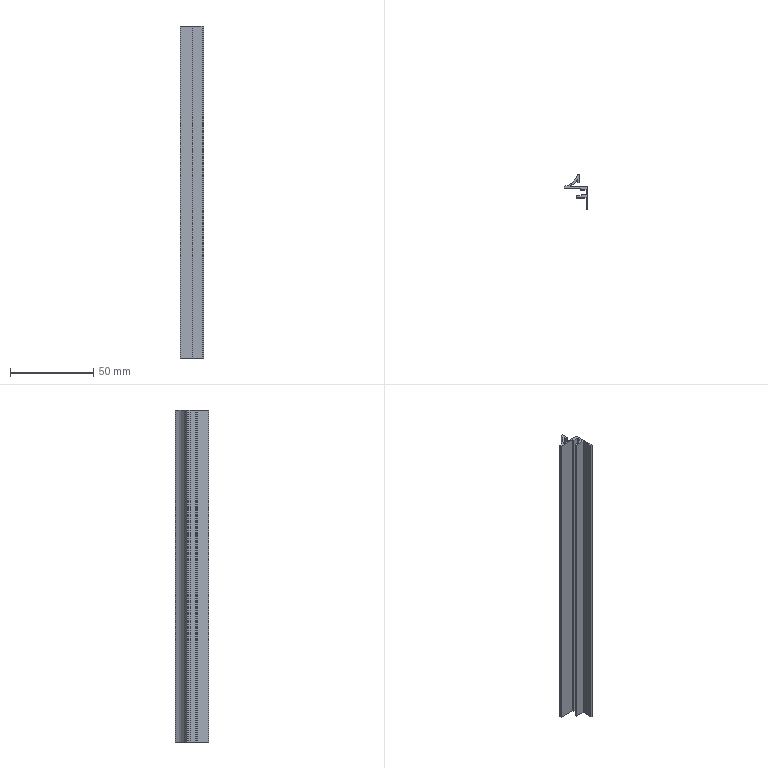Part | SolidWorks | features BaseBody 1, ICE 1, MoveFace 1 | 1 solid | 27 faces | box 14 x 20.3 x 199 mm | volume 10132 mm3 | plane 20 | cylinder 7 | commonest cylinder face diameters 0.387 x2 0.8 x2 0.4 x1 20 x1 22 x1
STEP:
#1=CARTESIAN_POINT('',(-5.304,-0.625,200.));
#2=VERTEX_POINT('',#1);
#3=CARTESIAN_POINT('',(-5.449,-0.8125,200.));
#4=VERTEX_POINT('',#3);
#5=CARTESIAN_POINT('',(-5.255,-0.8125,200.));
#6=DIRECTION('',(0.,0.,1.));
#7=DIRECTION('',(-1.,0.,0.));
#8=AXIS2_PLACEMENT_3D('',#5,#6,#7);
#9=CIRCLE('',#8,0.1937);
#10=EDGE_CURVE('',#2,#4,#9,.T.);
#11=ORIENTED_EDGE('',*,*,#10,.T.);
#12=CARTESIAN_POINT('',(-5.449,-0.8125,1.));
#13=VERTEX_POINT('',#12);
#14=CARTESIAN_POINT('',(-5.449,-0.8125,230.));
#15=DIRECTION('',(0.,0.,-1.));
#16=VECTOR('',#15,1000.);
#17=LINE('',#14,#16);
#18=EDGE_CURVE('',#4,#13,#17,.T.);
#19=ORIENTED_EDGE('',*,*,#18,.T.);
#20=CARTESIAN_POINT('',(-5.304,-0.625,1.));
#21=VERTEX_POINT('',#20);
#22=CARTESIAN_POINT('',(-5.255,-0.8125,1.));
#23=DIRECTION('',(0.,0.,-1.));
#24=DIRECTION('',(1.,0.,0.));
#25=AXIS2_PLACEMENT_3D('',#22,#23,#24);
#26=CIRCLE('',#25,0.1937);
#27=EDGE_CURVE('',#13,#21,#26,.T.);
#28=ORIENTED_EDGE('',*,*,#27,.T.);
#29=CARTESIAN_POINT('',(-5.304,-0.625,230.));
#30=DIRECTION('',(0.,0.,-1.));
#31=VECTOR('',#30,1000.);
#32=LINE('',#29,#31);
#33=EDGE_CURVE('',#2,#21,#32,.T.);
#34=ORIENTED_EDGE('',*,*,#33,.F.);
#35=EDGE_LOOP('',(#11,#19,#28,#34));
#36=FACE_OUTER_BOUND('',#35,.T.);
#37=CARTESIAN_POINT('',(-5.255,-0.8125,230.));
#38=DIRECTION('',(0.,0.,-1.));
#39=DIRECTION('',(-1.,0.,0.));
#40=AXIS2_PLACEMENT_3D('',#37,#38,#39);
#41=CYLINDRICAL_SURFACE('',#40,0.1937);
#42=ADVANCED_FACE('',(#36),#41,.F.);
#43=CARTESIAN_POINT('',(5.,-1.,1.));
#44=VERTEX_POINT('',#43);
#45=CARTESIAN_POINT('',(5.,-14.3,1.));
#46=VERTEX_POINT('',#45);
#47=CARTESIAN_POINT('',(5.,29.623,1.));
#48=DIRECTION('',(0.,-1.,0.));
#49=VECTOR('',#48,1000.);
#50=LINE('',#47,#49);
#51=EDGE_CURVE('',#44,#46,#50,.T.);
#52=ORIENTED_EDGE('',*,*,#51,.F.);
#53=CARTESIAN_POINT('',(5.,-1.,200.));
#54=VERTEX_POINT('',#53);
#55=CARTESIAN_POINT('',(5.,-1.,230.));
#56=DIRECTION('',(0.,0.,-1.));
#57=VECTOR('',#56,1000.);
#58=LINE('',#55,#57);
#59=EDGE_CURVE('',#54,#44,#58,.T.);
#60=ORIENTED_EDGE('',*,*,#59,.F.);
#61=CARTESIAN_POINT('',(5.,-14.3,200.));
#62=VERTEX_POINT('',#61);
#63=CARTESIAN_POINT('',(5.,-14.3,200.));
#64=DIRECTION('',(0.,1.,0.));
#65=VECTOR('',#64,1000.);
#66=LINE('',#63,#65);
#67=EDGE_CURVE('',#62,#54,#66,.T.);
#68=ORIENTED_EDGE('',*,*,#67,.F.);
#69=CARTESIAN_POINT('',(5.,-14.3,230.));
#70=DIRECTION('',(0.,0.,1.));
#71=VECTOR('',#70,1000.);
#72=LINE('',#69,#71);
#73=EDGE_CURVE('',#46,#62,#72,.T.);
#74=ORIENTED_EDGE('',*,*,#73,.F.);
#75=EDGE_LOOP('',(#52,#60,#68,#74));
#76=FACE_OUTER_BOUND('',#75,.T.);
#77=CARTESIAN_POINT('',(5.,-14.3,230.));
#78=DIRECTION('',(-1.,0.,0.));
#79=DIRECTION('',(0.,0.,1.));
#80=AXIS2_PLACEMENT_3D('',#77,#78,#79);
#81=PLANE('',#80);
#82=ADVANCED_FACE('',(#76),#81,.F.);
#83=CARTESIAN_POINT('',(-9.,-2.,1.));
#84=VERTEX_POINT('',#83);
#85=CARTESIAN_POINT('',(-9.,-2.,200.));
#86=VERTEX_POINT('',#85);
#87=CARTESIAN_POINT('',(-9.,-2.,230.));
#88=DIRECTION('',(0.,0.,1.));
#89=VECTOR('',#88,1000.);
#90=LINE('',#87,#89);
#91=EDGE_CURVE('',#84,#86,#90,.T.);
#92=ORIENTED_EDGE('',*,*,#91,.F.);
#93=CARTESIAN_POINT('',(0.9,-2.,1.));
#94=VERTEX_POINT('',#93);
#95=CARTESIAN_POINT('',(5.,-2.,1.));
#96=DIRECTION('',(-1.,0.,0.));
#97=VECTOR('',#96,1000.);
#98=LINE('',#95,#97);
#99=EDGE_CURVE('',#94,#84,#98,.T.);
#100=ORIENTED_EDGE('',*,*,#99,.F.);
#101=CARTESIAN_POINT('',(0.9,-2.,200.));
#102=VERTEX_POINT('',#101);
#103=CARTESIAN_POINT('',(0.9,-2.,230.));
#104=DIRECTION('',(0.,0.,-1.));
#105=VECTOR('',#104,1000.);
#106=LINE('',#103,#105);
#107=EDGE_CURVE('',#102,#94,#106,.T.);
#108=ORIENTED_EDGE('',*,*,#107,.F.);
#109=CARTESIAN_POINT('',(5.,-2.,200.));
#110=DIRECTION('',(1.,0.,0.));
#111=VECTOR('',#110,1000.);
#112=LINE('',#109,#111);
#113=EDGE_CURVE('',#86,#102,#112,.T.);
#114=ORIENTED_EDGE('',*,*,#113,.F.);
#115=EDGE_LOOP('',(#92,#100,#108,#114));
#116=FACE_OUTER_BOUND('',#115,.T.);
#117=CARTESIAN_POINT('',(-9.,-2.,230.));
#118=DIRECTION('',(0.,1.,0.));
#119=DIRECTION('',(0.,0.,1.));
#120=AXIS2_PLACEMENT_3D('',#117,#118,#119);
#121=PLANE('',#120);
#122=ADVANCED_FACE('',(#116),#121,.F.);
#123=CARTESIAN_POINT('',(4.,-6.,200.));
#124=VERTEX_POINT('',#123);
#125=CARTESIAN_POINT('',(4.,-3.,200.));
#126=VERTEX_POINT('',#125);
#127=CARTESIAN_POINT('',(4.,29.623,200.));
#128=DIRECTION('',(0.,1.,0.));
#129=VECTOR('',#128,1000.);
#130=LINE('',#127,#129);
#131=EDGE_CURVE('',#124,#126,#130,.T.);
#132=ORIENTED_EDGE('',*,*,#131,.F.);
#133=CARTESIAN_POINT('',(1.,-6.,200.));
#134=VERTEX_POINT('',#133);
#135=CARTESIAN_POINT('',(5.,-6.,200.));
#136=DIRECTION('',(1.,0.,0.));
#137=VECTOR('',#136,1000.);
#138=LINE('',#135,#137);
#139=EDGE_CURVE('',#134,#124,#138,.T.);
#140=ORIENTED_EDGE('',*,*,#139,.F.);
#141=CARTESIAN_POINT('',(1.,-6.7,200.));
#142=VERTEX_POINT('',#141);
#143=CARTESIAN_POINT('',(1.,-6.,200.));
#144=DIRECTION('',(0.,-1.,0.));
#145=VECTOR('',#144,1000.);
#146=LINE('',#143,#145);
#147=EDGE_CURVE('',#134,#142,#146,.T.);
#148=ORIENTED_EDGE('',*,*,#147,.T.);
#149=CARTESIAN_POINT('',(-1.7,-6.7,200.));
#150=VERTEX_POINT('',#149);
#151=CARTESIAN_POINT('',(5.,-6.7,200.));
#152=DIRECTION('',(1.,0.,0.));
#153=VECTOR('',#152,1000.);
#154=LINE('',#151,#153);
#155=EDGE_CURVE('',#150,#142,#154,.T.);
#156=ORIENTED_EDGE('',*,*,#155,.F.);
#157=CARTESIAN_POINT('',(-1.7,-7.7,200.));
#158=VERTEX_POINT('',#157);
#159=CARTESIAN_POINT('',(-1.7,-6.7,200.));
#160=DIRECTION('',(0.,-1.,0.));
#161=VECTOR('',#160,1000.);
#162=LINE('',#159,#161);
#163=EDGE_CURVE('',#150,#158,#162,.T.);
#164=ORIENTED_EDGE('',*,*,#163,.T.);
#165=CARTESIAN_POINT('',(4.,-7.7,200.));
#166=VERTEX_POINT('',#165);
#167=CARTESIAN_POINT('',(5.,-7.7,200.));
#168=DIRECTION('',(-1.,0.,0.));
#169=VECTOR('',#168,1000.);
#170=LINE('',#167,#169);
#171=EDGE_CURVE('',#166,#158,#170,.T.);
#172=ORIENTED_EDGE('',*,*,#171,.F.);
#173=CARTESIAN_POINT('',(4.,-14.3,200.));
#174=VERTEX_POINT('',#173);
#175=CARTESIAN_POINT('',(4.,29.623,200.));
#176=DIRECTION('',(0.,1.,0.));
#177=VECTOR('',#176,1000.);
#178=LINE('',#175,#177);
#179=EDGE_CURVE('',#174,#166,#178,.T.);
#180=ORIENTED_EDGE('',*,*,#179,.F.);
#181=CARTESIAN_POINT('',(5.,-14.3,200.));
#182=DIRECTION('',(-1.,0.,0.));
#183=VECTOR('',#182,1000.);
#184=LINE('',#181,#183);
#185=EDGE_CURVE('',#62,#174,#184,.T.);
#186=ORIENTED_EDGE('',*,*,#185,.F.);
#187=ORIENTED_EDGE('',*,*,#67,.T.);
#188=CARTESIAN_POINT('',(-5.207,-1.,200.));
#189=VERTEX_POINT('',#188);
#190=CARTESIAN_POINT('',(5.,-1.,200.));
#191=DIRECTION('',(1.,0.,0.));
#192=VECTOR('',#191,1000.);
#193=LINE('',#190,#192);
#194=EDGE_CURVE('',#189,#54,#193,.T.);
#195=ORIENTED_EDGE('',*,*,#194,.F.);
#196=CARTESIAN_POINT('',(-5.255,-0.8125,200.));
#197=DIRECTION('',(0.,0.,1.));
#198=DIRECTION('',(-1.,0.,0.));
#199=AXIS2_PLACEMENT_3D('',#196,#197,#198);
#200=CIRCLE('',#199,0.1937);
#201=EDGE_CURVE('',#4,#189,#200,.T.);
#202=ORIENTED_EDGE('',*,*,#201,.F.);
#203=ORIENTED_EDGE('',*,*,#10,.F.);
#204=CARTESIAN_POINT('',(-1.368,3.063,200.));
#205=VERTEX_POINT('',#204);
#206=CARTESIAN_POINT('',(-10.628,9.,200.));
#207=DIRECTION('',(0.,0.,1.));
#208=DIRECTION('',(-1.,0.,0.));
#209=AXIS2_PLACEMENT_3D('',#206,#207,#208);
#210=CIRCLE('',#209,11.);
#211=EDGE_CURVE('',#2,#205,#210,.T.);
#212=ORIENTED_EDGE('',*,*,#211,.T.);
#213=CARTESIAN_POINT('',(-1.,2.955,200.));
#214=VERTEX_POINT('',#213);
#215=CARTESIAN_POINT('',(-1.2,2.955,200.));
#216=DIRECTION('',(0.,0.,1.));
#217=DIRECTION('',(-1.,0.,0.));
#218=AXIS2_PLACEMENT_3D('',#215,#216,#217);
#219=CIRCLE('',#218,0.2);
#220=EDGE_CURVE('',#214,#205,#219,.T.);
#221=ORIENTED_EDGE('',*,*,#220,.F.);
#222=CARTESIAN_POINT('',(-1.,1.5,200.));
#223=VERTEX_POINT('',#222);
#224=CARTESIAN_POINT('',(-1.,2.955,200.));
#225=DIRECTION('',(0.,1.,0.));
#226=VECTOR('',#225,1000.);
#227=LINE('',#224,#226);
#228=EDGE_CURVE('',#223,#214,#227,.T.);
#229=ORIENTED_EDGE('',*,*,#228,.F.);
#230=CARTESIAN_POINT('',(0.,1.5,200.));
#231=VERTEX_POINT('',#230);
#232=CARTESIAN_POINT('',(-1.,1.5,200.));
#233=DIRECTION('',(-1.,0.,0.));
#234=VECTOR('',#233,1000.);
#235=LINE('',#232,#234);
#236=EDGE_CURVE('',#231,#223,#235,.T.);
#237=ORIENTED_EDGE('',*,*,#236,.F.);
#238=CARTESIAN_POINT('',(0.,6.,200.));
#239=VERTEX_POINT('',#238);
#240=CARTESIAN_POINT('',(0.,1.5,200.));
#241=DIRECTION('',(0.,-1.,0.));
#242=VECTOR('',#241,1000.);
#243=LINE('',#240,#242);
#244=EDGE_CURVE('',#239,#231,#243,.T.);
#245=ORIENTED_EDGE('',*,*,#244,.F.);
#246=CARTESIAN_POINT('',(-0.8,6.,200.));
#247=VERTEX_POINT('',#246);
#248=CARTESIAN_POINT('',(0.,6.,200.));
#249=DIRECTION('',(1.,0.,0.));
#250=VECTOR('',#249,1000.);
#251=LINE('',#248,#250);
#252=EDGE_CURVE('',#247,#239,#251,.T.);
#253=ORIENTED_EDGE('',*,*,#252,.F.);
#254=CARTESIAN_POINT('',(-1.178,5.731,200.));
#255=VERTEX_POINT('',#254);
#256=CARTESIAN_POINT('',(-0.8,5.6,200.));
#257=DIRECTION('',(0.,0.,1.));
#258=DIRECTION('',(-1.,0.,0.));
#259=AXIS2_PLACEMENT_3D('',#256,#257,#258);
#260=CIRCLE('',#259,0.4);
#261=EDGE_CURVE('',#247,#255,#260,.T.);
#262=ORIENTED_EDGE('',*,*,#261,.T.);
#263=CARTESIAN_POINT('',(-8.678,-0.8077,200.));
#264=VERTEX_POINT('',#263);
#265=CARTESIAN_POINT('',(-10.628,9.,200.));
#266=DIRECTION('',(0.,0.,1.));
#267=DIRECTION('',(-1.,0.,0.));
#268=AXIS2_PLACEMENT_3D('',#265,#266,#267);
#269=CIRCLE('',#268,10.);
#270=EDGE_CURVE('',#264,#255,#269,.T.);
#271=ORIENTED_EDGE('',*,*,#270,.F.);
#272=CARTESIAN_POINT('',(-9.,-1.2,200.));
#273=VERTEX_POINT('',#272);
#274=CARTESIAN_POINT('',(-8.6,-1.2,200.));
#275=DIRECTION('',(0.,0.,1.));
#276=DIRECTION('',(-1.,0.,0.));
#277=AXIS2_PLACEMENT_3D('',#274,#275,#276);
#278=CIRCLE('',#277,0.4);
#279=EDGE_CURVE('',#264,#273,#278,.T.);
#280=ORIENTED_EDGE('',*,*,#279,.T.);
#281=CARTESIAN_POINT('',(-9.,8.,200.));
#282=DIRECTION('',(0.,-1.,0.));
#283=VECTOR('',#282,1000.);
#284=LINE('',#281,#283);
#285=EDGE_CURVE('',#273,#86,#284,.T.);
#286=ORIENTED_EDGE('',*,*,#285,.T.);
#287=ORIENTED_EDGE('',*,*,#113,.T.);
#288=CARTESIAN_POINT('',(0.9,-3.,200.));
#289=VERTEX_POINT('',#288);
#290=CARTESIAN_POINT('',(0.9,29.623,200.));
#291=DIRECTION('',(0.,1.,0.));
#292=VECTOR('',#291,1000.);
#293=LINE('',#290,#292);
#294=EDGE_CURVE('',#289,#102,#293,.T.);
#295=ORIENTED_EDGE('',*,*,#294,.F.);
#296=CARTESIAN_POINT('',(5.,-3.,200.));
#297=DIRECTION('',(-1.,0.,0.));
#298=VECTOR('',#297,1000.);
#299=LINE('',#296,#298);
#300=EDGE_CURVE('',#126,#289,#299,.T.);
#301=ORIENTED_EDGE('',*,*,#300,.F.);
#302=EDGE_LOOP('',(#132,#140,#148,#156,#164,#172,#180,#186,#187,#195,#202,#203,#212,#221,#229,#237,#245,#253,#262,#271,#280,#286,#287,#295,#301));
#303=FACE_OUTER_BOUND('',#302,.T.);
#304=CARTESIAN_POINT('',(5.,29.623,200.));
#305=DIRECTION('',(0.,0.,-1.));
#306=DIRECTION('',(-1.,0.,0.));
#307=AXIS2_PLACEMENT_3D('',#304,#305,#306);
#308=PLANE('',#307);
#309=ADVANCED_FACE('',(#303),#308,.F.);
#310=ORIENTED_EDGE('',*,*,#185,.T.);
#311=CARTESIAN_POINT('',(4.,-14.3,1.));
#312=VERTEX_POINT('',#311);
#313=CARTESIAN_POINT('',(4.,-14.3,230.));
#314=DIRECTION('',(0.,0.,1.));
#315=VECTOR('',#314,1000.);
#316=LINE('',#313,#315);
#317=EDGE_CURVE('',#312,#174,#316,.T.);
#318=ORIENTED_EDGE('',*,*,#317,.F.);
#319=CARTESIAN_POINT('',(5.,-14.3,1.));
#320=DIRECTION('',(-1.,0.,0.));
#321=VECTOR('',#320,1000.);
#322=LINE('',#319,#321);
#323=EDGE_CURVE('',#46,#312,#322,.T.);
#324=ORIENTED_EDGE('',*,*,#323,.F.);
#325=ORIENTED_EDGE('',*,*,#73,.T.);
#326=EDGE_LOOP('',(#310,#318,#324,#325));
#327=FACE_OUTER_BOUND('',#326,.T.);
#328=CARTESIAN_POINT('',(4.,-14.3,230.));
#329=DIRECTION('',(0.,1.,0.));
#330=DIRECTION('',(0.,0.,1.));
#331=AXIS2_PLACEMENT_3D('',#328,#329,#330);
#332=PLANE('',#331);
#333=ADVANCED_FACE('',(#327),#332,.F.);
#334=ORIENTED_EDGE('',*,*,#51,.T.);
#335=ORIENTED_EDGE('',*,*,#323,.T.);
#336=CARTESIAN_POINT('',(4.,-7.7,1.));
#337=VERTEX_POINT('',#336);
#338=CARTESIAN_POINT('',(4.,-7.7,1.));
#339=DIRECTION('',(0.,-1.,0.));
#340=VECTOR('',#339,1000.);
#341=LINE('',#338,#340);
#342=EDGE_CURVE('',#337,#312,#341,.T.);
#343=ORIENTED_EDGE('',*,*,#342,.F.);
#344=CARTESIAN_POINT('',(-1.7,-7.7,1.));
#345=VERTEX_POINT('',#344);
#346=CARTESIAN_POINT('',(-1.7,-7.7,1.));
#347=DIRECTION('',(1.,0.,0.));
#348=VECTOR('',#347,1000.);
#349=LINE('',#346,#348);
#350=EDGE_CURVE('',#345,#337,#349,.T.);
#351=ORIENTED_EDGE('',*,*,#350,.F.);
#352=CARTESIAN_POINT('',(-1.7,-6.7,1.));
#353=VERTEX_POINT('',#352);
#354=CARTESIAN_POINT('',(-1.7,29.623,1.));
#355=DIRECTION('',(0.,1.,0.));
#356=VECTOR('',#355,1000.);
#357=LINE('',#354,#356);
#358=EDGE_CURVE('',#345,#353,#357,.T.);
#359=ORIENTED_EDGE('',*,*,#358,.T.);
#360=CARTESIAN_POINT('',(1.,-6.7,1.));
#361=VERTEX_POINT('',#360);
#362=CARTESIAN_POINT('',(1.,-6.7,1.));
#363=DIRECTION('',(-1.,0.,0.));
#364=VECTOR('',#363,1000.);
#365=LINE('',#362,#364);
#366=EDGE_CURVE('',#361,#353,#365,.T.);
#367=ORIENTED_EDGE('',*,*,#366,.F.);
#368=CARTESIAN_POINT('',(1.,-6.,1.));
#369=VERTEX_POINT('',#368);
#370=CARTESIAN_POINT('',(1.,29.623,1.));
#371=DIRECTION('',(0.,1.,0.));
#372=VECTOR('',#371,1000.);
#373=LINE('',#370,#372);
#374=EDGE_CURVE('',#361,#369,#373,.T.);
#375=ORIENTED_EDGE('',*,*,#374,.T.);
#376=CARTESIAN_POINT('',(4.,-6.,1.));
#377=VERTEX_POINT('',#376);
#378=CARTESIAN_POINT('',(4.,-6.,1.));
#379=DIRECTION('',(-1.,0.,0.));
#380=VECTOR('',#379,1000.);
#381=LINE('',#378,#380);
#382=EDGE_CURVE('',#377,#369,#381,.T.);
#383=ORIENTED_EDGE('',*,*,#382,.F.);
#384=CARTESIAN_POINT('',(4.,-3.,1.));
#385=VERTEX_POINT('',#384);
#386=CARTESIAN_POINT('',(4.,-3.,1.));
#387=DIRECTION('',(0.,-1.,0.));
#388=VECTOR('',#387,1000.);
#389=LINE('',#386,#388);
#390=EDGE_CURVE('',#385,#377,#389,.T.);
#391=ORIENTED_EDGE('',*,*,#390,.F.);
#392=CARTESIAN_POINT('',(0.9,-3.,1.));
#393=VERTEX_POINT('',#392);
#394=CARTESIAN_POINT('',(0.9,-3.,1.));
#395=DIRECTION('',(1.,0.,0.));
#396=VECTOR('',#395,1000.);
#397=LINE('',#394,#396);
#398=EDGE_CURVE('',#393,#385,#397,.T.);
#399=ORIENTED_EDGE('',*,*,#398,.F.);
#400=CARTESIAN_POINT('',(0.9,-2.,1.));
#401=DIRECTION('',(0.,-1.,0.));
#402=VECTOR('',#401,1000.);
#403=LINE('',#400,#402);
#404=EDGE_CURVE('',#94,#393,#403,.T.);
#405=ORIENTED_EDGE('',*,*,#404,.F.);
#406=ORIENTED_EDGE('',*,*,#99,.T.);
#407=CARTESIAN_POINT('',(-9.,-1.2,1.));
#408=VERTEX_POINT('',#407);
#409=CARTESIAN_POINT('',(-9.,-1.2,1.));
#410=DIRECTION('',(0.,-1.,0.));
#411=VECTOR('',#410,1000.);
#412=LINE('',#409,#411);
#413=EDGE_CURVE('',#408,#84,#412,.T.);
#414=ORIENTED_EDGE('',*,*,#413,.F.);
#415=CARTESIAN_POINT('',(-8.678,-0.8077,1.));
#416=VERTEX_POINT('',#415);
#417=CARTESIAN_POINT('',(-8.6,-1.2,1.));
#418=DIRECTION('',(0.,0.,-1.));
#419=DIRECTION('',(1.,0.,0.));
#420=AXIS2_PLACEMENT_3D('',#417,#418,#419);
#421=CIRCLE('',#420,0.4);
#422=EDGE_CURVE('',#408,#416,#421,.T.);
#423=ORIENTED_EDGE('',*,*,#422,.T.);
#424=CARTESIAN_POINT('',(-1.178,5.731,1.));
#425=VERTEX_POINT('',#424);
#426=CARTESIAN_POINT('',(-10.628,9.,1.));
#427=DIRECTION('',(0.,0.,-1.));
#428=DIRECTION('',(1.,0.,0.));
#429=AXIS2_PLACEMENT_3D('',#426,#427,#428);
#430=CIRCLE('',#429,10.);
#431=EDGE_CURVE('',#425,#416,#430,.T.);
#432=ORIENTED_EDGE('',*,*,#431,.F.);
#433=CARTESIAN_POINT('',(-0.8,6.,1.));
#434=VERTEX_POINT('',#433);
#435=CARTESIAN_POINT('',(-0.8,5.6,1.));
#436=DIRECTION('',(0.,0.,-1.));
#437=DIRECTION('',(1.,0.,0.));
#438=AXIS2_PLACEMENT_3D('',#435,#436,#437);
#439=CIRCLE('',#438,0.4);
#440=EDGE_CURVE('',#425,#434,#439,.T.);
#441=ORIENTED_EDGE('',*,*,#440,.T.);
#442=CARTESIAN_POINT('',(0.,6.,1.));
#443=VERTEX_POINT('',#442);
#444=CARTESIAN_POINT('',(0.,6.,1.));
#445=DIRECTION('',(-1.,0.,0.));
#446=VECTOR('',#445,1000.);
#447=LINE('',#444,#446);
#448=EDGE_CURVE('',#443,#434,#447,.T.);
#449=ORIENTED_EDGE('',*,*,#448,.F.);
#450=CARTESIAN_POINT('',(0.,1.5,1.));
#451=VERTEX_POINT('',#450);
#452=CARTESIAN_POINT('',(0.,1.5,1.));
#453=DIRECTION('',(0.,1.,0.));
#454=VECTOR('',#453,1000.);
#455=LINE('',#452,#454);
#456=EDGE_CURVE('',#451,#443,#455,.T.);
#457=ORIENTED_EDGE('',*,*,#456,.F.);
#458=CARTESIAN_POINT('',(-1.,1.5,1.));
#459=VERTEX_POINT('',#458);
#460=CARTESIAN_POINT('',(-1.,1.5,1.));
#461=DIRECTION('',(1.,0.,0.));
#462=VECTOR('',#461,1000.);
#463=LINE('',#460,#462);
#464=EDGE_CURVE('',#459,#451,#463,.T.);
#465=ORIENTED_EDGE('',*,*,#464,.F.);
#466=CARTESIAN_POINT('',(-1.,2.955,1.));
#467=VERTEX_POINT('',#466);
#468=CARTESIAN_POINT('',(-1.,2.955,1.));
#469=DIRECTION('',(0.,-1.,0.));
#470=VECTOR('',#469,1000.);
#471=LINE('',#468,#470);
#472=EDGE_CURVE('',#467,#459,#471,.T.);
#473=ORIENTED_EDGE('',*,*,#472,.F.);
#474=CARTESIAN_POINT('',(-1.368,3.063,1.));
#475=VERTEX_POINT('',#474);
#476=CARTESIAN_POINT('',(-1.2,2.955,1.));
#477=DIRECTION('',(0.,0.,-1.));
#478=DIRECTION('',(1.,0.,0.));
#479=AXIS2_PLACEMENT_3D('',#476,#477,#478);
#480=CIRCLE('',#479,0.2);
#481=EDGE_CURVE('',#475,#467,#480,.T.);
#482=ORIENTED_EDGE('',*,*,#481,.F.);
#483=CARTESIAN_POINT('',(-10.628,9.,1.));
#484=DIRECTION('',(0.,0.,-1.));
#485=DIRECTION('',(1.,0.,0.));
#486=AXIS2_PLACEMENT_3D('',#483,#484,#485);
#487=CIRCLE('',#486,11.);
#488=EDGE_CURVE('',#475,#21,#487,.T.);
#489=ORIENTED_EDGE('',*,*,#488,.T.);
#490=ORIENTED_EDGE('',*,*,#27,.F.);
#491=CARTESIAN_POINT('',(-5.207,-1.,1.));
#492=VERTEX_POINT('',#491);
#493=CARTESIAN_POINT('',(-5.255,-0.8125,1.));
#494=DIRECTION('',(0.,0.,-1.));
#495=DIRECTION('',(1.,0.,0.));
#496=AXIS2_PLACEMENT_3D('',#493,#494,#495);
#497=CIRCLE('',#496,0.1937);
#498=EDGE_CURVE('',#492,#13,#497,.T.);
#499=ORIENTED_EDGE('',*,*,#498,.F.);
#500=CARTESIAN_POINT('',(5.,-1.,1.));
#501=DIRECTION('',(-1.,0.,0.));
#502=VECTOR('',#501,1000.);
#503=LINE('',#500,#502);
#504=EDGE_CURVE('',#44,#492,#503,.T.);
#505=ORIENTED_EDGE('',*,*,#504,.F.);
#506=EDGE_LOOP('',(#334,#335,#343,#351,#359,#367,#375,#383,#391,#399,#405,#406,#414,#423,#432,#441,#449,#457,#465,#473,#482,#489,#490,#499,#505));
#507=FACE_OUTER_BOUND('',#506,.T.);
#508=CARTESIAN_POINT('',(5.,29.623,1.));
#509=DIRECTION('',(0.,0.,1.));
#510=DIRECTION('',(1.,0.,0.));
#511=AXIS2_PLACEMENT_3D('',#508,#509,#510);
#512=PLANE('',#511);
#513=ADVANCED_FACE('',(#507),#512,.F.);
#514=ORIENTED_EDGE('',*,*,#59,.T.);
#515=ORIENTED_EDGE('',*,*,#504,.T.);
#516=CARTESIAN_POINT('',(-5.207,-1.,230.));
#517=DIRECTION('',(0.,0.,-1.));
#518=VECTOR('',#517,1000.);
#519=LINE('',#516,#518);
#520=EDGE_CURVE('',#189,#492,#519,.T.);
#521=ORIENTED_EDGE('',*,*,#520,.F.);
#522=ORIENTED_EDGE('',*,*,#194,.T.);
#523=EDGE_LOOP('',(#514,#515,#521,#522));
#524=FACE_OUTER_BOUND('',#523,.T.);
#525=CARTESIAN_POINT('',(5.,-1.,230.));
#526=DIRECTION('',(0.,-1.,0.));
#527=DIRECTION('',(0.,0.,-1.));
#528=AXIS2_PLACEMENT_3D('',#525,#526,#527);
#529=PLANE('',#528);
#530=ADVANCED_FACE('',(#524),#529,.F.);
#531=CARTESIAN_POINT('',(-9.,-1.2,230.));
#532=DIRECTION('',(0.,0.,1.));
#533=VECTOR('',#532,1000.);
#534=LINE('',#531,#533);
#535=EDGE_CURVE('',#408,#273,#534,.T.);
#536=ORIENTED_EDGE('',*,*,#535,.F.);
#537=ORIENTED_EDGE('',*,*,#413,.T.);
#538=ORIENTED_EDGE('',*,*,#91,.T.);
#539=ORIENTED_EDGE('',*,*,#285,.F.);
#540=EDGE_LOOP('',(#536,#537,#538,#539));
#541=FACE_OUTER_BOUND('',#540,.T.);
#542=CARTESIAN_POINT('',(-9.,-1.2,230.));
#543=DIRECTION('',(1.,0.,0.));
#544=DIRECTION('',(0.,0.,-1.));
#545=AXIS2_PLACEMENT_3D('',#542,#543,#544);
#546=PLANE('',#545);
#547=ADVANCED_FACE('',(#541),#546,.F.);
#548=ORIENTED_EDGE('',*,*,#294,.T.);
#549=ORIENTED_EDGE('',*,*,#107,.T.);
#550=ORIENTED_EDGE('',*,*,#404,.T.);
#551=CARTESIAN_POINT('',(0.9,-3.,230.));
#552=DIRECTION('',(0.,0.,-1.));
#553=VECTOR('',#552,1000.);
#554=LINE('',#551,#553);
#555=EDGE_CURVE('',#289,#393,#554,.T.);
#556=ORIENTED_EDGE('',*,*,#555,.F.);
#557=EDGE_LOOP('',(#548,#549,#550,#556));
#558=FACE_OUTER_BOUND('',#557,.T.);
#559=CARTESIAN_POINT('',(0.9,-2.,230.));
#560=DIRECTION('',(1.,0.,0.));
#561=DIRECTION('',(0.,0.,-1.));
#562=AXIS2_PLACEMENT_3D('',#559,#560,#561);
#563=PLANE('',#562);
#564=ADVANCED_FACE('',(#558),#563,.F.);
#565=ORIENTED_EDGE('',*,*,#300,.T.);
#566=ORIENTED_EDGE('',*,*,#555,.T.);
#567=ORIENTED_EDGE('',*,*,#398,.T.);
#568=CARTESIAN_POINT('',(4.,-3.,230.));
#569=DIRECTION('',(0.,0.,-1.));
#570=VECTOR('',#569,1000.);
#571=LINE('',#568,#570);
#572=EDGE_CURVE('',#126,#385,#571,.T.);
#573=ORIENTED_EDGE('',*,*,#572,.F.);
#574=EDGE_LOOP('',(#565,#566,#567,#573));
#575=FACE_OUTER_BOUND('',#574,.T.);
#576=CARTESIAN_POINT('',(0.9,-3.,230.));
#577=DIRECTION('',(0.,1.,0.));
#578=DIRECTION('',(0.,0.,1.));
#579=AXIS2_PLACEMENT_3D('',#576,#577,#578);
#580=PLANE('',#579);
#581=ADVANCED_FACE('',(#575),#580,.F.);
#582=ORIENTED_EDGE('',*,*,#131,.T.);
#583=ORIENTED_EDGE('',*,*,#572,.T.);
#584=ORIENTED_EDGE('',*,*,#390,.T.);
#585=CARTESIAN_POINT('',(4.,-6.,230.));
#586=DIRECTION('',(0.,0.,-1.));
#587=VECTOR('',#586,1000.);
#588=LINE('',#585,#587);
#589=EDGE_CURVE('',#124,#377,#588,.T.);
#590=ORIENTED_EDGE('',*,*,#589,.F.);
#591=EDGE_LOOP('',(#582,#583,#584,#590));
#592=FACE_OUTER_BOUND('',#591,.T.);
#593=CARTESIAN_POINT('',(4.,-3.,230.));
#594=DIRECTION('',(1.,0.,0.));
#595=DIRECTION('',(0.,0.,-1.));
#596=AXIS2_PLACEMENT_3D('',#593,#594,#595);
#597=PLANE('',#596);
#598=ADVANCED_FACE('',(#592),#597,.F.);
#599=ORIENTED_EDGE('',*,*,#139,.T.);
#600=ORIENTED_EDGE('',*,*,#589,.T.);
#601=ORIENTED_EDGE('',*,*,#382,.T.);
#602=CARTESIAN_POINT('',(1.,-6.,230.));
#603=DIRECTION('',(0.,0.,-1.));
#604=VECTOR('',#603,1000.);
#605=LINE('',#602,#604);
#606=EDGE_CURVE('',#134,#369,#605,.T.);
#607=ORIENTED_EDGE('',*,*,#606,.F.);
#608=EDGE_LOOP('',(#599,#600,#601,#607));
#609=FACE_OUTER_BOUND('',#608,.T.);
#610=CARTESIAN_POINT('',(4.,-6.,230.));
#611=DIRECTION('',(0.,-1.,0.));
#612=DIRECTION('',(0.,0.,-1.));
#613=AXIS2_PLACEMENT_3D('',#610,#611,#612);
#614=PLANE('',#613);
#615=ADVANCED_FACE('',(#609),#614,.F.);
#616=ORIENTED_EDGE('',*,*,#155,.T.);
#617=CARTESIAN_POINT('',(1.,-6.7,230.));
#618=DIRECTION('',(0.,0.,1.));
#619=VECTOR('',#618,1000.);
#620=LINE('',#617,#619);
#621=EDGE_CURVE('',#361,#142,#620,.T.);
#622=ORIENTED_EDGE('',*,*,#621,.F.);
#623=ORIENTED_EDGE('',*,*,#366,.T.);
#624=CARTESIAN_POINT('',(-1.7,-6.7,230.));
#625=DIRECTION('',(0.,0.,-1.));
#626=VECTOR('',#625,1000.);
#627=LINE('',#624,#626);
#628=EDGE_CURVE('',#150,#353,#627,.T.);
#629=ORIENTED_EDGE('',*,*,#628,.F.);
#630=EDGE_LOOP('',(#616,#622,#623,#629));
#631=FACE_OUTER_BOUND('',#630,.T.);
#632=CARTESIAN_POINT('',(1.,-6.7,230.));
#633=DIRECTION('',(0.,-1.,0.));
#634=DIRECTION('',(0.,0.,-1.));
#635=AXIS2_PLACEMENT_3D('',#632,#633,#634);
#636=PLANE('',#635);
#637=ADVANCED_FACE('',(#631),#636,.F.);
#638=ORIENTED_EDGE('',*,*,#171,.T.);
#639=CARTESIAN_POINT('',(-1.7,-7.7,230.));
#640=DIRECTION('',(0.,0.,1.));
#641=VECTOR('',#640,1000.);
#642=LINE('',#639,#641);
#643=EDGE_CURVE('',#345,#158,#642,.T.);
#644=ORIENTED_EDGE('',*,*,#643,.F.);
#645=ORIENTED_EDGE('',*,*,#350,.T.);
#646=CARTESIAN_POINT('',(4.,-7.7,230.));
#647=DIRECTION('',(0.,0.,-1.));
#648=VECTOR('',#647,1000.);
#649=LINE('',#646,#648);
#650=EDGE_CURVE('',#166,#337,#649,.T.);
#651=ORIENTED_EDGE('',*,*,#650,.F.);
#652=EDGE_LOOP('',(#638,#644,#645,#651));
#653=FACE_OUTER_BOUND('',#652,.T.);
#654=CARTESIAN_POINT('',(-1.7,-7.7,230.));
#655=DIRECTION('',(0.,1.,0.));
#656=DIRECTION('',(0.,0.,1.));
#657=AXIS2_PLACEMENT_3D('',#654,#655,#656);
#658=PLANE('',#657);
#659=ADVANCED_FACE('',(#653),#658,.F.);
#660=ORIENTED_EDGE('',*,*,#179,.T.);
#661=ORIENTED_EDGE('',*,*,#650,.T.);
#662=ORIENTED_EDGE('',*,*,#342,.T.);
#663=ORIENTED_EDGE('',*,*,#317,.T.);
#664=EDGE_LOOP('',(#660,#661,#662,#663));
#665=FACE_OUTER_BOUND('',#664,.T.);
#666=CARTESIAN_POINT('',(4.,-7.7,230.));
#667=DIRECTION('',(1.,0.,0.));
#668=DIRECTION('',(0.,0.,-1.));
#669=AXIS2_PLACEMENT_3D('',#666,#667,#668);
#670=PLANE('',#669);
#671=ADVANCED_FACE('',(#665),#670,.F.);
#672=ORIENTED_EDGE('',*,*,#18,.F.);
#673=ORIENTED_EDGE('',*,*,#201,.T.);
#674=ORIENTED_EDGE('',*,*,#520,.T.);
#675=ORIENTED_EDGE('',*,*,#498,.T.);
#676=EDGE_LOOP('',(#672,#673,#674,#675));
#677=FACE_OUTER_BOUND('',#676,.T.);
#678=CARTESIAN_POINT('',(-5.255,-0.8125,230.));
#679=DIRECTION('',(0.,0.,-1.));
#680=DIRECTION('',(-1.,0.,0.));
#681=AXIS2_PLACEMENT_3D('',#678,#679,#680);
#682=CYLINDRICAL_SURFACE('',#681,0.1937);
#683=ADVANCED_FACE('',(#677),#682,.F.);
#684=CARTESIAN_POINT('',(-1.,2.955,230.));
#685=DIRECTION('',(0.,0.,1.));
#686=VECTOR('',#685,1000.);
#687=LINE('',#684,#686);
#688=EDGE_CURVE('',#467,#214,#687,.T.);
#689=ORIENTED_EDGE('',*,*,#688,.F.);
#690=ORIENTED_EDGE('',*,*,#472,.T.);
#691=CARTESIAN_POINT('',(-1.,1.5,230.));
#692=DIRECTION('',(0.,0.,-1.));
#693=VECTOR('',#692,1000.);
#694=LINE('',#691,#693);
#695=EDGE_CURVE('',#223,#459,#694,.T.);
#696=ORIENTED_EDGE('',*,*,#695,.F.);
#697=ORIENTED_EDGE('',*,*,#228,.T.);
#698=EDGE_LOOP('',(#689,#690,#696,#697));
#699=FACE_OUTER_BOUND('',#698,.T.);
#700=CARTESIAN_POINT('',(-1.,2.955,230.));
#701=DIRECTION('',(1.,0.,0.));
#702=DIRECTION('',(0.,0.,-1.));
#703=AXIS2_PLACEMENT_3D('',#700,#701,#702);
#704=PLANE('',#703);
#705=ADVANCED_FACE('',(#699),#704,.F.);
#706=ORIENTED_EDGE('',*,*,#488,.F.);
#707=CARTESIAN_POINT('',(-1.368,3.063,230.));
#708=DIRECTION('',(0.,0.,1.));
#709=VECTOR('',#708,1000.);
#710=LINE('',#707,#709);
#711=EDGE_CURVE('',#475,#205,#710,.T.);
#712=ORIENTED_EDGE('',*,*,#711,.T.);
#713=ORIENTED_EDGE('',*,*,#211,.F.);
#714=ORIENTED_EDGE('',*,*,#33,.T.);
#715=EDGE_LOOP('',(#706,#712,#713,#714));
#716=FACE_OUTER_BOUND('',#715,.T.);
#717=CARTESIAN_POINT('',(-10.628,9.,230.));
#718=DIRECTION('',(0.,0.,-1.));
#719=DIRECTION('',(-1.,0.,0.));
#720=AXIS2_PLACEMENT_3D('',#717,#718,#719);
#721=CYLINDRICAL_SURFACE('',#720,11.);
#722=ADVANCED_FACE('',(#716),#721,.T.);
#723=CARTESIAN_POINT('',(-1.178,5.731,230.));
#724=DIRECTION('',(0.,0.,1.));
#725=VECTOR('',#724,1000.);
#726=LINE('',#723,#725);
#727=EDGE_CURVE('',#425,#255,#726,.T.);
#728=ORIENTED_EDGE('',*,*,#727,.F.);
#729=ORIENTED_EDGE('',*,*,#431,.T.);
#730=CARTESIAN_POINT('',(-8.678,-0.8077,230.));
#731=DIRECTION('',(0.,0.,-1.));
#732=VECTOR('',#731,1000.);
#733=LINE('',#730,#732);
#734=EDGE_CURVE('',#264,#416,#733,.T.);
#735=ORIENTED_EDGE('',*,*,#734,.F.);
#736=ORIENTED_EDGE('',*,*,#270,.T.);
#737=EDGE_LOOP('',(#728,#729,#735,#736));
#738=FACE_OUTER_BOUND('',#737,.T.);
#739=CARTESIAN_POINT('',(-10.628,9.,230.));
#740=DIRECTION('',(0.,0.,-1.));
#741=DIRECTION('',(-1.,0.,0.));
#742=AXIS2_PLACEMENT_3D('',#739,#740,#741);
#743=CYLINDRICAL_SURFACE('',#742,10.);
#744=ADVANCED_FACE('',(#738),#743,.F.);
#745=CARTESIAN_POINT('',(0.,1.5,230.));
#746=DIRECTION('',(0.,0.,1.));
#747=VECTOR('',#746,1000.);
#748=LINE('',#745,#747);
#749=EDGE_CURVE('',#451,#231,#748,.T.);
#750=ORIENTED_EDGE('',*,*,#749,.F.);
#751=ORIENTED_EDGE('',*,*,#456,.T.);
#752=CARTESIAN_POINT('',(0.,6.,230.));
#753=DIRECTION('',(0.,0.,-1.));
#754=VECTOR('',#753,1000.);
#755=LINE('',#752,#754);
#756=EDGE_CURVE('',#239,#443,#755,.T.);
#757=ORIENTED_EDGE('',*,*,#756,.F.);
#758=ORIENTED_EDGE('',*,*,#244,.T.);
#759=EDGE_LOOP('',(#750,#751,#757,#758));
#760=FACE_OUTER_BOUND('',#759,.T.);
#761=CARTESIAN_POINT('',(0.,1.5,230.));
#762=DIRECTION('',(-1.,0.,0.));
#763=DIRECTION('',(0.,0.,1.));
#764=AXIS2_PLACEMENT_3D('',#761,#762,#763);
#765=PLANE('',#764);
#766=ADVANCED_FACE('',(#760),#765,.F.);
#767=ORIENTED_EDGE('',*,*,#422,.F.);
#768=ORIENTED_EDGE('',*,*,#535,.T.);
#769=ORIENTED_EDGE('',*,*,#279,.F.);
#770=ORIENTED_EDGE('',*,*,#734,.T.);
#771=EDGE_LOOP('',(#767,#768,#769,#770));
#772=FACE_OUTER_BOUND('',#771,.T.);
#773=CARTESIAN_POINT('',(-8.6,-1.2,230.));
#774=DIRECTION('',(0.,0.,-1.));
#775=DIRECTION('',(-1.,0.,0.));
#776=AXIS2_PLACEMENT_3D('',#773,#774,#775);
#777=CYLINDRICAL_SURFACE('',#776,0.4);
#778=ADVANCED_FACE('',(#772),#777,.T.);
#779=ORIENTED_EDGE('',*,*,#147,.F.);
#780=ORIENTED_EDGE('',*,*,#606,.T.);
#781=ORIENTED_EDGE('',*,*,#374,.F.);
#782=ORIENTED_EDGE('',*,*,#621,.T.);
#783=EDGE_LOOP('',(#779,#780,#781,#782));
#784=FACE_OUTER_BOUND('',#783,.T.);
#785=CARTESIAN_POINT('',(1.,-6.,230.));
#786=DIRECTION('',(1.,0.,0.));
#787=DIRECTION('',(0.,0.,-1.));
#788=AXIS2_PLACEMENT_3D('',#785,#786,#787);
#789=PLANE('',#788);
#790=ADVANCED_FACE('',(#784),#789,.F.);
#791=ORIENTED_EDGE('',*,*,#163,.F.);
#792=ORIENTED_EDGE('',*,*,#628,.T.);
#793=ORIENTED_EDGE('',*,*,#358,.F.);
#794=ORIENTED_EDGE('',*,*,#643,.T.);
#795=EDGE_LOOP('',(#791,#792,#793,#794));
#796=FACE_OUTER_BOUND('',#795,.T.);
#797=CARTESIAN_POINT('',(-1.7,-6.7,230.));
#798=DIRECTION('',(1.,0.,0.));
#799=DIRECTION('',(0.,0.,-1.));
#800=AXIS2_PLACEMENT_3D('',#797,#798,#799);
#801=PLANE('',#800);
#802=ADVANCED_FACE('',(#796),#801,.F.);
#803=ORIENTED_EDGE('',*,*,#711,.F.);
#804=ORIENTED_EDGE('',*,*,#481,.T.);
#805=ORIENTED_EDGE('',*,*,#688,.T.);
#806=ORIENTED_EDGE('',*,*,#220,.T.);
#807=EDGE_LOOP('',(#803,#804,#805,#806));
#808=FACE_OUTER_BOUND('',#807,.T.);
#809=CARTESIAN_POINT('',(-1.2,2.955,230.));
#810=DIRECTION('',(0.,0.,-1.));
#811=DIRECTION('',(-1.,0.,0.));
#812=AXIS2_PLACEMENT_3D('',#809,#810,#811);
#813=CYLINDRICAL_SURFACE('',#812,0.2);
#814=ADVANCED_FACE('',(#808),#813,.F.);
#815=ORIENTED_EDGE('',*,*,#695,.T.);
#816=ORIENTED_EDGE('',*,*,#464,.T.);
#817=ORIENTED_EDGE('',*,*,#749,.T.);
#818=ORIENTED_EDGE('',*,*,#236,.T.);
#819=EDGE_LOOP('',(#815,#816,#817,#818));
#820=FACE_OUTER_BOUND('',#819,.T.);
#821=CARTESIAN_POINT('',(-1.,1.5,230.));
#822=DIRECTION('',(0.,1.,0.));
#823=DIRECTION('',(0.,0.,1.));
#824=AXIS2_PLACEMENT_3D('',#821,#822,#823);
#825=PLANE('',#824);
#826=ADVANCED_FACE('',(#820),#825,.F.);
#827=ORIENTED_EDGE('',*,*,#440,.F.);
#828=ORIENTED_EDGE('',*,*,#727,.T.);
#829=ORIENTED_EDGE('',*,*,#261,.F.);
#830=CARTESIAN_POINT('',(-0.8,6.,230.));
#831=DIRECTION('',(0.,0.,-1.));
#832=VECTOR('',#831,1000.);
#833=LINE('',#830,#832);
#834=EDGE_CURVE('',#247,#434,#833,.T.);
#835=ORIENTED_EDGE('',*,*,#834,.T.);
#836=EDGE_LOOP('',(#827,#828,#829,#835));
#837=FACE_OUTER_BOUND('',#836,.T.);
#838=CARTESIAN_POINT('',(-0.8,5.6,230.));
#839=DIRECTION('',(0.,0.,-1.));
#840=DIRECTION('',(-1.,0.,0.));
#841=AXIS2_PLACEMENT_3D('',#838,#839,#840);
#842=CYLINDRICAL_SURFACE('',#841,0.4);
#843=ADVANCED_FACE('',(#837),#842,.T.);
#844=ORIENTED_EDGE('',*,*,#756,.T.);
#845=ORIENTED_EDGE('',*,*,#448,.T.);
#846=ORIENTED_EDGE('',*,*,#834,.F.);
#847=ORIENTED_EDGE('',*,*,#252,.T.);
#848=EDGE_LOOP('',(#844,#845,#846,#847));
#849=FACE_OUTER_BOUND('',#848,.T.);
#850=CARTESIAN_POINT('',(0.,6.,230.));
#851=DIRECTION('',(0.,-1.,0.));
#852=DIRECTION('',(0.,0.,-1.));
#853=AXIS2_PLACEMENT_3D('',#850,#851,#852);
#854=PLANE('',#853);
#855=ADVANCED_FACE('',(#849),#854,.F.);
#856=CLOSED_SHELL('',(#42,#82,#122,#309,#333,#513,#530,#547,#564,#581,#598,#615,#637,#659,#671,#683,#705,#722,#744,#766,#778,#790,#802,#814,#826,#843,#855));
#857=MANIFOLD_SOLID_BREP('',#856);
#858=CARTESIAN_POINT('',(0.,0.,0.));
#859=DIRECTION('',(0.,0.,1.));
#860=DIRECTION('',(1.,0.,0.));
#861=AXIS2_PLACEMENT_3D('',#858,#859,#860);
#862=(LENGTH_UNIT()NAMED_UNIT(*)SI_UNIT(.MILLI.,.METRE.));
#863=UNCERTAINTY_MEASURE_WITH_UNIT(LENGTH_MEASURE(0.00001),#862,'','');
#864=(NAMED_UNIT(*)PLANE_ANGLE_UNIT()SI_UNIT($,.RADIAN.));
#865=(NAMED_UNIT(*)SI_UNIT($,.STERADIAN.)SOLID_ANGLE_UNIT());
#866=(GEOMETRIC_REPRESENTATION_CONTEXT(3)GLOBAL_UNCERTAINTY_ASSIGNED_CONTEXT((#863))GLOBAL_UNIT_ASSIGNED_CONTEXT((#862,#864,#865))REPRESENTATION_CONTEXT('',''));
#867=ADVANCED_BREP_SHAPE_REPRESENTATION('',(#857,#861),#866);